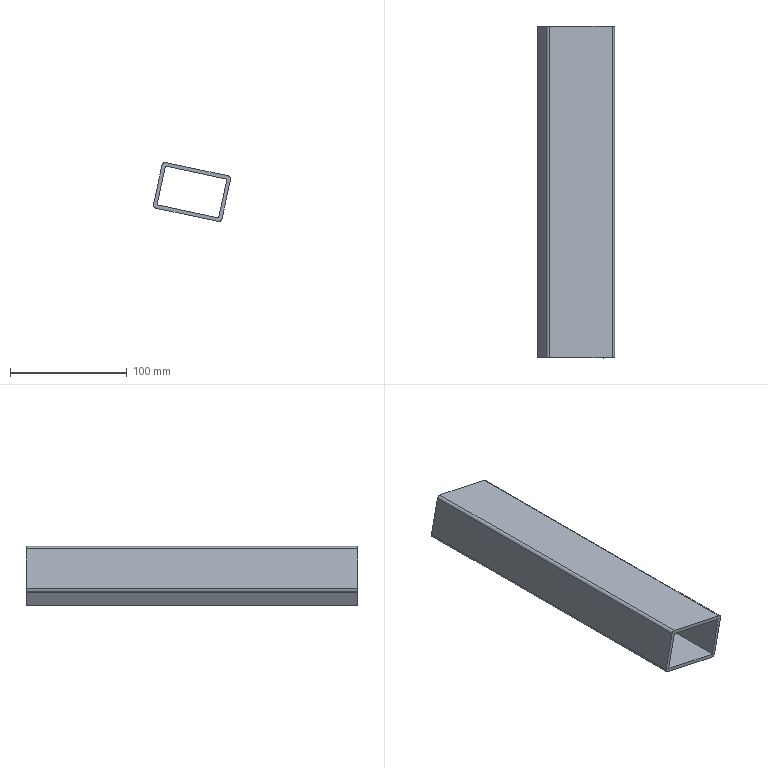Part | STEP file | support fixing frame | 1 solid | 14 faces | box 66.075 x 284.5 x 50.67 mm | volume 158932 mm3 | plane 10 | cylinder 4 | commonest cylinder face diameters 5 x4
STEP:
#1=CARTESIAN_POINT('',(0.,0.,0.));
#2=DIRECTION('',(0.,0.,1.));
#3=DIRECTION('',(1.,0.,0.));
#4=AXIS2_PLACEMENT_3D('',#1,#2,#3);
#5=CARTESIAN_POINT('',(1767.422,305.,-292.036));
#6=VERTEX_POINT('',#5);
#7=CARTESIAN_POINT('',(1770.387,305.,-290.111));
#8=VERTEX_POINT('',#7);
#9=CARTESIAN_POINT('',(1769.867,305.,-292.556));
#10=DIRECTION('',(0.,1.,0.));
#11=DIRECTION('',(0.,0.,-1.));
#12=AXIS2_PLACEMENT_3D('',#9,#10,#11);
#13=CIRCLE('',#12,2.5);
#14=CARTESIAN_POINT('',(1769.867,0.,-292.556));
#15=DIRECTION('',(0.,1.,0.));
#16=DIRECTION('',(1.,0.,0.));
#17=AXIS2_PLACEMENT_3D('',#14,#15,#16);
#18=CYLINDRICAL_SURFACE('',#17,2.5);
#19=CARTESIAN_POINT('',(1.571,305.));
#20=DIRECTION('',(1.,0.));
#21=VECTOR('',#20,1.);
#22=LINE('',#19,#21);
#23=(GEOMETRIC_REPRESENTATION_CONTEXT(2)PARAMETRIC_REPRESENTATION_CONTEXT()REPRESENTATION_CONTEXT('',''));
#24=DEFINITIONAL_REPRESENTATION('',(#22),#23);
#25=PCURVE('',#18,#24);
#26=CARTESIAN_POINT('',(1655.76,305.,323.083));
#27=DIRECTION('',(0.,-1.,0.));
#28=DIRECTION('',(0.,0.,1.));
#29=AXIS2_PLACEMENT_3D('',#26,#27,#28);
#30=PLANE('',#29);
#31=CARTESIAN_POINT('',(-618.139,-114.107));
#32=CARTESIAN_POINT('',(-618.139,-109.777));
#33=CARTESIAN_POINT('',(-614.389,-111.942));
#34=CARTESIAN_POINT('',(-610.639,-114.107));
#35=CARTESIAN_POINT('',(-614.389,-116.272));
#36=CARTESIAN_POINT('',(-618.139,-118.437));
#37=CARTESIAN_POINT('',(-618.139,-114.107));
#38=(BOUNDED_CURVE()B_SPLINE_CURVE(2,(#31,#32,#33,#34,#35,#36,#37),.UNSPECIFIED.,.T.,.F.)B_SPLINE_CURVE_WITH_KNOTS((1,2,2,2,2,1),(-2.094,0.,2.094,4.189,6.283,8.378),.UNSPECIFIED.)CURVE()GEOMETRIC_REPRESENTATION_ITEM()RATIONAL_B_SPLINE_CURVE((1.,0.5,1.,0.5,1.,0.5,1.))REPRESENTATION_ITEM(''));
#39=(GEOMETRIC_REPRESENTATION_CONTEXT(2)PARAMETRIC_REPRESENTATION_CONTEXT()REPRESENTATION_CONTEXT('',''));
#40=DEFINITIONAL_REPRESENTATION('',(#38),#39);
#41=PCURVE('',#30,#40);
#42=SURFACE_CURVE('',#13,(#25,#41),.PCURVE_S1.);
#43=EDGE_CURVE('',#6,#8,#42,.T.);
#44=ORIENTED_EDGE('',*,*,#43,.F.);
#45=CARTESIAN_POINT('',(1767.422,20.5,-292.036));
#46=VERTEX_POINT('',#45);
#47=CARTESIAN_POINT('',(1767.422,386.,-292.036));
#48=DIRECTION('',(0.,1.,0.));
#49=VECTOR('',#48,1.);
#50=LINE('',#47,#49);
#51=CARTESIAN_POINT('',(3.351,386.));
#52=DIRECTION('',(0.,1.));
#53=VECTOR('',#52,1.);
#54=LINE('',#51,#53);
#55=(GEOMETRIC_REPRESENTATION_CONTEXT(2)PARAMETRIC_REPRESENTATION_CONTEXT()REPRESENTATION_CONTEXT('',''));
#56=DEFINITIONAL_REPRESENTATION('',(#54),#55);
#57=PCURVE('',#18,#56);
#58=CARTESIAN_POINT('',(1767.941,386.,-289.591));
#59=DIRECTION('',(0.9781,0.,-0.2079));
#60=DIRECTION('',(0.2079,0.,0.9781));
#61=AXIS2_PLACEMENT_3D('',#58,#59,#60);
#62=PLANE('',#61);
#63=CARTESIAN_POINT('',(-2.5,0.));
#64=DIRECTION('',(0.,-1.));
#65=VECTOR('',#64,1.);
#66=LINE('',#63,#65);
#67=(GEOMETRIC_REPRESENTATION_CONTEXT(2)PARAMETRIC_REPRESENTATION_CONTEXT()REPRESENTATION_CONTEXT('',''));
#68=DEFINITIONAL_REPRESENTATION('',(#66),#67);
#69=PCURVE('',#62,#68);
#70=SURFACE_CURVE('',#50,(#57,#69),.PCURVE_S1.);
#71=EDGE_CURVE('',#46,#6,#70,.T.);
#72=ORIENTED_EDGE('',*,*,#71,.F.);
#73=CARTESIAN_POINT('',(1770.387,20.5,-290.111));
#74=VERTEX_POINT('',#73);
#75=CARTESIAN_POINT('',(1769.867,20.5,-292.556));
#76=DIRECTION('',(0.,-1.,0.));
#77=DIRECTION('',(-1.,0.,0.));
#78=AXIS2_PLACEMENT_3D('',#75,#76,#77);
#79=CIRCLE('',#78,2.5);
#80=CARTESIAN_POINT('',(9.425,20.5));
#81=DIRECTION('',(-1.,0.));
#82=VECTOR('',#81,1.);
#83=LINE('',#80,#82);
#84=(GEOMETRIC_REPRESENTATION_CONTEXT(2)PARAMETRIC_REPRESENTATION_CONTEXT()REPRESENTATION_CONTEXT('',''));
#85=DEFINITIONAL_REPRESENTATION('',(#83),#84);
#86=PCURVE('',#18,#85);
#87=CARTESIAN_POINT('',(1767.941,20.5,-289.591));
#88=DIRECTION('',(0.,1.,0.));
#89=DIRECTION('',(1.,0.,0.));
#90=AXIS2_PLACEMENT_3D('',#87,#88,#89);
#91=PLANE('',#90);
#92=CARTESIAN_POINT('',(-0.5744,2.965));
#93=CARTESIAN_POINT('',(-0.5744,7.295));
#94=CARTESIAN_POINT('',(3.176,5.13));
#95=CARTESIAN_POINT('',(6.926,2.965));
#96=CARTESIAN_POINT('',(3.176,0.8001));
#97=CARTESIAN_POINT('',(-0.5744,-1.365));
#98=CARTESIAN_POINT('',(-0.5744,2.965));
#99=(BOUNDED_CURVE()B_SPLINE_CURVE(2,(#92,#93,#94,#95,#96,#97,#98),.UNSPECIFIED.,.T.,.F.)B_SPLINE_CURVE_WITH_KNOTS((1,2,2,2,2,1),(-2.094,0.,2.094,4.189,6.283,8.378),.UNSPECIFIED.)CURVE()GEOMETRIC_REPRESENTATION_ITEM()RATIONAL_B_SPLINE_CURVE((1.,0.5,1.,0.5,1.,0.5,1.))REPRESENTATION_ITEM(''));
#100=(GEOMETRIC_REPRESENTATION_CONTEXT(2)PARAMETRIC_REPRESENTATION_CONTEXT()REPRESENTATION_CONTEXT('',''));
#101=DEFINITIONAL_REPRESENTATION('',(#99),#100);
#102=PCURVE('',#91,#101);
#103=SURFACE_CURVE('',#79,(#86,#102),.PCURVE_S1.);
#104=EDGE_CURVE('',#74,#46,#103,.T.);
#105=ORIENTED_EDGE('',*,*,#104,.F.);
#106=CARTESIAN_POINT('',(1770.387,20.5,-290.111));
#107=DIRECTION('',(0.,-1.,0.));
#108=VECTOR('',#107,1.);
#109=LINE('',#106,#108);
#110=CARTESIAN_POINT('',(4.922,20.5));
#111=DIRECTION('',(0.,-1.));
#112=VECTOR('',#111,1.);
#113=LINE('',#110,#112);
#114=(GEOMETRIC_REPRESENTATION_CONTEXT(2)PARAMETRIC_REPRESENTATION_CONTEXT()REPRESENTATION_CONTEXT('',''));
#115=DEFINITIONAL_REPRESENTATION('',(#113),#114);
#116=PCURVE('',#18,#115);
#117=CARTESIAN_POINT('',(17.53,0.,82.471));
#118=DIRECTION('',(0.2079,0.,0.9781));
#119=DIRECTION('',(-0.9781,0.,0.2079));
#120=AXIS2_PLACEMENT_3D('',#117,#118,#119);
#121=PLANE('',#120);
#122=CARTESIAN_POINT('',(-1792.017,-20.5));
#123=DIRECTION('',(0.,1.));
#124=VECTOR('',#123,1.);
#125=LINE('',#122,#124);
#126=(GEOMETRIC_REPRESENTATION_CONTEXT(2)PARAMETRIC_REPRESENTATION_CONTEXT()REPRESENTATION_CONTEXT('',''));
#127=DEFINITIONAL_REPRESENTATION('',(#125),#126);
#128=PCURVE('',#121,#127);
#129=SURFACE_CURVE('',#109,(#116,#128),.PCURVE_S1.);
#130=EDGE_CURVE('',#8,#74,#129,.T.);
#131=ORIENTED_EDGE('',*,*,#130,.F.);
#132=EDGE_LOOP('',(#44,#72,#105,#131));
#133=FACE_BOUND('',#132,.T.);
#134=ADVANCED_FACE('',(#133),#18,.T.);
#135=CARTESIAN_POINT('',(1826.11,20.5,-304.511));
#136=VERTEX_POINT('',#135);
#137=CARTESIAN_POINT('',(1824.185,20.5,-301.546));
#138=VERTEX_POINT('',#137);
#139=CARTESIAN_POINT('',(1823.665,20.5,-303.991));
#140=DIRECTION('',(0.,-1.,0.));
#141=DIRECTION('',(-1.,0.,0.));
#142=AXIS2_PLACEMENT_3D('',#139,#140,#141);
#143=CIRCLE('',#142,2.5);
#144=CARTESIAN_POINT('',(1823.665,0.,-303.991));
#145=DIRECTION('',(0.,-1.,0.));
#146=DIRECTION('',(0.,0.,1.));
#147=AXIS2_PLACEMENT_3D('',#144,#145,#146);
#148=CYLINDRICAL_SURFACE('',#147,2.5);
#149=CARTESIAN_POINT('',(1.571,-20.5));
#150=DIRECTION('',(1.,0.));
#151=VECTOR('',#150,1.);
#152=LINE('',#149,#151);
#153=(GEOMETRIC_REPRESENTATION_CONTEXT(2)PARAMETRIC_REPRESENTATION_CONTEXT()REPRESENTATION_CONTEXT('',''));
#154=DEFINITIONAL_REPRESENTATION('',(#152),#153);
#155=PCURVE('',#148,#154);
#156=CARTESIAN_POINT('',(53.224,14.4));
#157=CARTESIAN_POINT('',(53.224,18.73));
#158=CARTESIAN_POINT('',(56.974,16.565));
#159=CARTESIAN_POINT('',(60.724,14.4));
#160=CARTESIAN_POINT('',(56.974,12.235));
#161=CARTESIAN_POINT('',(53.224,10.07));
#162=CARTESIAN_POINT('',(53.224,14.4));
#163=(BOUNDED_CURVE()B_SPLINE_CURVE(2,(#156,#157,#158,#159,#160,#161,#162),.UNSPECIFIED.,.T.,.F.)B_SPLINE_CURVE_WITH_KNOTS((1,2,2,2,2,1),(-2.094,0.,2.094,4.189,6.283,8.378),.UNSPECIFIED.)CURVE()GEOMETRIC_REPRESENTATION_ITEM()RATIONAL_B_SPLINE_CURVE((1.,0.5,1.,0.5,1.,0.5,1.))REPRESENTATION_ITEM(''));
#164=(GEOMETRIC_REPRESENTATION_CONTEXT(2)PARAMETRIC_REPRESENTATION_CONTEXT()REPRESENTATION_CONTEXT('',''));
#165=DEFINITIONAL_REPRESENTATION('',(#163),#164);
#166=PCURVE('',#91,#165);
#167=SURFACE_CURVE('',#143,(#155,#166),.PCURVE_S1.);
#168=EDGE_CURVE('',#136,#138,#167,.T.);
#169=ORIENTED_EDGE('',*,*,#168,.F.);
#170=CARTESIAN_POINT('',(1826.11,305.,-304.511));
#171=VERTEX_POINT('',#170);
#172=CARTESIAN_POINT('',(1826.11,20.5,-304.511));
#173=DIRECTION('',(0.,-1.,0.));
#174=VECTOR('',#173,1.);
#175=LINE('',#172,#174);
#176=CARTESIAN_POINT('',(4.503,-20.5));
#177=DIRECTION('',(0.,1.));
#178=VECTOR('',#177,1.);
#179=LINE('',#176,#178);
#180=(GEOMETRIC_REPRESENTATION_CONTEXT(2)PARAMETRIC_REPRESENTATION_CONTEXT()REPRESENTATION_CONTEXT('',''));
#181=DEFINITIONAL_REPRESENTATION('',(#179),#180);
#182=PCURVE('',#148,#181);
#183=CARTESIAN_POINT('',(1826.63,20.5,-302.066));
#184=DIRECTION('',(-0.9781,0.,0.2079));
#185=DIRECTION('',(-0.2079,0.,-0.9781));
#186=AXIS2_PLACEMENT_3D('',#183,#184,#185);
#187=PLANE('',#186);
#188=CARTESIAN_POINT('',(2.5,0.));
#189=DIRECTION('',(0.,1.));
#190=VECTOR('',#189,1.);
#191=LINE('',#188,#190);
#192=(GEOMETRIC_REPRESENTATION_CONTEXT(2)PARAMETRIC_REPRESENTATION_CONTEXT()REPRESENTATION_CONTEXT('',''));
#193=DEFINITIONAL_REPRESENTATION('',(#191),#192);
#194=PCURVE('',#187,#193);
#195=SURFACE_CURVE('',#175,(#182,#194),.PCURVE_S1.);
#196=EDGE_CURVE('',#171,#136,#195,.T.);
#197=ORIENTED_EDGE('',*,*,#196,.F.);
#198=CARTESIAN_POINT('',(1824.185,305.,-301.546));
#199=VERTEX_POINT('',#198);
#200=CARTESIAN_POINT('',(1823.665,305.,-303.991));
#201=DIRECTION('',(0.,1.,0.));
#202=DIRECTION('',(0.,0.,-1.));
#203=AXIS2_PLACEMENT_3D('',#200,#201,#202);
#204=CIRCLE('',#203,2.5);
#205=CARTESIAN_POINT('',(9.425,-305.));
#206=DIRECTION('',(-1.,0.));
#207=VECTOR('',#206,1.);
#208=LINE('',#205,#207);
#209=(GEOMETRIC_REPRESENTATION_CONTEXT(2)PARAMETRIC_REPRESENTATION_CONTEXT()REPRESENTATION_CONTEXT('',''));
#210=DEFINITIONAL_REPRESENTATION('',(#208),#209);
#211=PCURVE('',#148,#210);
#212=CARTESIAN_POINT('',(-629.574,-167.905));
#213=CARTESIAN_POINT('',(-629.574,-163.575));
#214=CARTESIAN_POINT('',(-625.824,-165.74));
#215=CARTESIAN_POINT('',(-622.074,-167.905));
#216=CARTESIAN_POINT('',(-625.824,-170.07));
#217=CARTESIAN_POINT('',(-629.574,-172.235));
#218=CARTESIAN_POINT('',(-629.574,-167.905));
#219=(BOUNDED_CURVE()B_SPLINE_CURVE(2,(#212,#213,#214,#215,#216,#217,#218),.UNSPECIFIED.,.T.,.F.)B_SPLINE_CURVE_WITH_KNOTS((1,2,2,2,2,1),(-2.094,0.,2.094,4.189,6.283,8.378),.UNSPECIFIED.)CURVE()GEOMETRIC_REPRESENTATION_ITEM()RATIONAL_B_SPLINE_CURVE((1.,0.5,1.,0.5,1.,0.5,1.))REPRESENTATION_ITEM(''));
#220=(GEOMETRIC_REPRESENTATION_CONTEXT(2)PARAMETRIC_REPRESENTATION_CONTEXT()REPRESENTATION_CONTEXT('',''));
#221=DEFINITIONAL_REPRESENTATION('',(#219),#220);
#222=PCURVE('',#30,#221);
#223=SURFACE_CURVE('',#204,(#211,#222),.PCURVE_S1.);
#224=EDGE_CURVE('',#199,#171,#223,.T.);
#225=ORIENTED_EDGE('',*,*,#224,.F.);
#226=CARTESIAN_POINT('',(1824.185,386.,-301.546));
#227=DIRECTION('',(0.,1.,0.));
#228=VECTOR('',#227,1.);
#229=LINE('',#226,#228);
#230=CARTESIAN_POINT('',(6.074,-386.));
#231=DIRECTION('',(0.,-1.));
#232=VECTOR('',#231,1.);
#233=LINE('',#230,#232);
#234=(GEOMETRIC_REPRESENTATION_CONTEXT(2)PARAMETRIC_REPRESENTATION_CONTEXT()REPRESENTATION_CONTEXT('',''));
#235=DEFINITIONAL_REPRESENTATION('',(#233),#234);
#236=PCURVE('',#148,#235);
#237=CARTESIAN_POINT('',(-1847.017,-386.));
#238=DIRECTION('',(0.,-1.));
#239=VECTOR('',#238,1.);
#240=LINE('',#237,#239);
#241=(GEOMETRIC_REPRESENTATION_CONTEXT(2)PARAMETRIC_REPRESENTATION_CONTEXT()REPRESENTATION_CONTEXT('',''));
#242=DEFINITIONAL_REPRESENTATION('',(#240),#241);
#243=PCURVE('',#121,#242);
#244=SURFACE_CURVE('',#229,(#236,#243),.PCURVE_S1.);
#245=EDGE_CURVE('',#138,#199,#244,.T.);
#246=ORIENTED_EDGE('',*,*,#245,.F.);
#247=EDGE_LOOP('',(#169,#197,#225,#246));
#248=FACE_BOUND('',#247,.T.);
#249=ADVANCED_FACE('',(#248),#148,.T.);
#250=CARTESIAN_POINT('',(1762.07,305.,-329.237));
#251=VERTEX_POINT('',#250);
#252=CARTESIAN_POINT('',(1760.145,305.,-326.271));
#253=VERTEX_POINT('',#252);
#254=CARTESIAN_POINT('',(1762.59,305.,-326.791));
#255=DIRECTION('',(0.,1.,0.));
#256=DIRECTION('',(0.,0.,-1.));
#257=AXIS2_PLACEMENT_3D('',#254,#255,#256);
#258=CIRCLE('',#257,2.5);
#259=CARTESIAN_POINT('',(1762.59,386.,-326.791));
#260=DIRECTION('',(0.,-1.,0.));
#261=DIRECTION('',(-1.,0.,0.));
#262=AXIS2_PLACEMENT_3D('',#259,#260,#261);
#263=CYLINDRICAL_SURFACE('',#262,2.5);
#264=CARTESIAN_POINT('',(1.571,81.));
#265=DIRECTION('',(-1.,0.));
#266=VECTOR('',#265,1.);
#267=LINE('',#264,#266);
#268=(GEOMETRIC_REPRESENTATION_CONTEXT(2)PARAMETRIC_REPRESENTATION_CONTEXT()REPRESENTATION_CONTEXT('',''));
#269=DEFINITIONAL_REPRESENTATION('',(#267),#268);
#270=PCURVE('',#263,#269);
#271=CARTESIAN_POINT('',(-652.374,-106.83));
#272=CARTESIAN_POINT('',(-652.374,-102.5));
#273=CARTESIAN_POINT('',(-648.624,-104.665));
#274=CARTESIAN_POINT('',(-644.874,-106.83));
#275=CARTESIAN_POINT('',(-648.624,-108.995));
#276=CARTESIAN_POINT('',(-652.374,-111.16));
#277=CARTESIAN_POINT('',(-652.374,-106.83));
#278=(BOUNDED_CURVE()B_SPLINE_CURVE(2,(#271,#272,#273,#274,#275,#276,#277),.UNSPECIFIED.,.T.,.F.)B_SPLINE_CURVE_WITH_KNOTS((1,2,2,2,2,1),(-2.094,0.,2.094,4.189,6.283,8.378),.UNSPECIFIED.)CURVE()GEOMETRIC_REPRESENTATION_ITEM()RATIONAL_B_SPLINE_CURVE((1.,0.5,1.,0.5,1.,0.5,1.))REPRESENTATION_ITEM(''));
#279=(GEOMETRIC_REPRESENTATION_CONTEXT(2)PARAMETRIC_REPRESENTATION_CONTEXT()REPRESENTATION_CONTEXT('',''));
#280=DEFINITIONAL_REPRESENTATION('',(#278),#279);
#281=PCURVE('',#30,#280);
#282=SURFACE_CURVE('',#258,(#270,#281),.PCURVE_S1.);
#283=EDGE_CURVE('',#251,#253,#282,.T.);
#284=ORIENTED_EDGE('',*,*,#283,.F.);
#285=CARTESIAN_POINT('',(1762.07,20.5,-329.237));
#286=VERTEX_POINT('',#285);
#287=CARTESIAN_POINT('',(1762.07,0.,-329.237));
#288=DIRECTION('',(0.,1.,0.));
#289=VECTOR('',#288,1.);
#290=LINE('',#287,#289);
#291=CARTESIAN_POINT('',(1.361,386.));
#292=DIRECTION('',(0.,-1.));
#293=VECTOR('',#292,1.);
#294=LINE('',#291,#293);
#295=(GEOMETRIC_REPRESENTATION_CONTEXT(2)PARAMETRIC_REPRESENTATION_CONTEXT()REPRESENTATION_CONTEXT('',''));
#296=DEFINITIONAL_REPRESENTATION('',(#294),#295);
#297=PCURVE('',#263,#296);
#298=CARTESIAN_POINT('',(9.213,0.,43.345));
#299=DIRECTION('',(0.2079,0.,0.9781));
#300=DIRECTION('',(-0.9781,0.,0.2079));
#301=AXIS2_PLACEMENT_3D('',#298,#299,#300);
#302=PLANE('',#301);
#303=CARTESIAN_POINT('',(-1792.017,0.));
#304=DIRECTION('',(0.,-1.));
#305=VECTOR('',#304,1.);
#306=LINE('',#303,#305);
#307=(GEOMETRIC_REPRESENTATION_CONTEXT(2)PARAMETRIC_REPRESENTATION_CONTEXT()REPRESENTATION_CONTEXT('',''));
#308=DEFINITIONAL_REPRESENTATION('',(#306),#307);
#309=PCURVE('',#302,#308);
#310=SURFACE_CURVE('',#290,(#297,#309),.PCURVE_S1.);
#311=EDGE_CURVE('',#286,#251,#310,.T.);
#312=ORIENTED_EDGE('',*,*,#311,.F.);
#313=CARTESIAN_POINT('',(1760.145,20.5,-326.271));
#314=VERTEX_POINT('',#313);
#315=CARTESIAN_POINT('',(1762.59,20.5,-326.791));
#316=DIRECTION('',(0.,-1.,0.));
#317=DIRECTION('',(-1.,0.,0.));
#318=AXIS2_PLACEMENT_3D('',#315,#316,#317);
#319=CIRCLE('',#318,2.5);
#320=CARTESIAN_POINT('',(-6.283,365.5));
#321=DIRECTION('',(1.,0.));
#322=VECTOR('',#321,1.);
#323=LINE('',#320,#322);
#324=(GEOMETRIC_REPRESENTATION_CONTEXT(2)PARAMETRIC_REPRESENTATION_CONTEXT()REPRESENTATION_CONTEXT('',''));
#325=DEFINITIONAL_REPRESENTATION('',(#323),#324);
#326=PCURVE('',#263,#325);
#327=CARTESIAN_POINT('',(-7.851,37.2));
#328=CARTESIAN_POINT('',(-7.851,41.53));
#329=CARTESIAN_POINT('',(-4.101,39.365));
#330=CARTESIAN_POINT('',(-0.3513,37.2));
#331=CARTESIAN_POINT('',(-4.101,35.035));
#332=CARTESIAN_POINT('',(-7.851,32.87));
#333=CARTESIAN_POINT('',(-7.851,37.2));
#334=(BOUNDED_CURVE()B_SPLINE_CURVE(2,(#327,#328,#329,#330,#331,#332,#333),.UNSPECIFIED.,.T.,.F.)B_SPLINE_CURVE_WITH_KNOTS((1,2,2,2,2,1),(-2.094,0.,2.094,4.189,6.283,8.378),.UNSPECIFIED.)CURVE()GEOMETRIC_REPRESENTATION_ITEM()RATIONAL_B_SPLINE_CURVE((1.,0.5,1.,0.5,1.,0.5,1.))REPRESENTATION_ITEM(''));
#335=(GEOMETRIC_REPRESENTATION_CONTEXT(2)PARAMETRIC_REPRESENTATION_CONTEXT()REPRESENTATION_CONTEXT('',''));
#336=DEFINITIONAL_REPRESENTATION('',(#334),#335);
#337=PCURVE('',#91,#336);
#338=SURFACE_CURVE('',#319,(#326,#337),.PCURVE_S1.);
#339=EDGE_CURVE('',#314,#286,#338,.T.);
#340=ORIENTED_EDGE('',*,*,#339,.F.);
#341=CARTESIAN_POINT('',(1760.145,386.,-326.271));
#342=DIRECTION('',(0.,-1.,0.));
#343=VECTOR('',#342,1.);
#344=LINE('',#341,#343);
#345=CARTESIAN_POINT('',(-0.2094,0.));
#346=DIRECTION('',(0.,1.));
#347=VECTOR('',#346,1.);
#348=LINE('',#345,#347);
#349=(GEOMETRIC_REPRESENTATION_CONTEXT(2)PARAMETRIC_REPRESENTATION_CONTEXT()REPRESENTATION_CONTEXT('',''));
#350=DEFINITIONAL_REPRESENTATION('',(#348),#349);
#351=PCURVE('',#263,#350);
#352=CARTESIAN_POINT('',(-37.5,0.));
#353=DIRECTION('',(0.,1.));
#354=VECTOR('',#353,1.);
#355=LINE('',#352,#354);
#356=(GEOMETRIC_REPRESENTATION_CONTEXT(2)PARAMETRIC_REPRESENTATION_CONTEXT()REPRESENTATION_CONTEXT('',''));
#357=DEFINITIONAL_REPRESENTATION('',(#355),#356);
#358=PCURVE('',#62,#357);
#359=SURFACE_CURVE('',#344,(#351,#358),.PCURVE_S1.);
#360=EDGE_CURVE('',#253,#314,#359,.T.);
#361=ORIENTED_EDGE('',*,*,#360,.F.);
#362=EDGE_LOOP('',(#284,#312,#340,#361));
#363=FACE_BOUND('',#362,.T.);
#364=ADVANCED_FACE('',(#363),#263,.T.);
#365=CARTESIAN_POINT('',(1815.868,20.5,-340.672));
#366=VERTEX_POINT('',#365);
#367=CARTESIAN_POINT('',(1818.833,20.5,-338.746));
#368=VERTEX_POINT('',#367);
#369=CARTESIAN_POINT('',(1816.388,20.5,-338.226));
#370=DIRECTION('',(0.,-1.,0.));
#371=DIRECTION('',(-1.,0.,0.));
#372=AXIS2_PLACEMENT_3D('',#369,#370,#371);
#373=CIRCLE('',#372,2.5);
#374=CARTESIAN_POINT('',(1816.388,20.5,-338.226));
#375=DIRECTION('',(0.,1.,0.));
#376=DIRECTION('',(0.,0.,-1.));
#377=AXIS2_PLACEMENT_3D('',#374,#375,#376);
#378=CYLINDRICAL_SURFACE('',#377,2.5);
#379=CARTESIAN_POINT('',(7.854,0.));
#380=DIRECTION('',(-1.,0.));
#381=VECTOR('',#380,1.);
#382=LINE('',#379,#381);
#383=(GEOMETRIC_REPRESENTATION_CONTEXT(2)PARAMETRIC_REPRESENTATION_CONTEXT()REPRESENTATION_CONTEXT('',''));
#384=DEFINITIONAL_REPRESENTATION('',(#382),#383);
#385=PCURVE('',#378,#384);
#386=CARTESIAN_POINT('',(45.947,48.635));
#387=CARTESIAN_POINT('',(45.947,52.966));
#388=CARTESIAN_POINT('',(49.697,50.801));
#389=CARTESIAN_POINT('',(53.447,48.635));
#390=CARTESIAN_POINT('',(49.697,46.47));
#391=CARTESIAN_POINT('',(45.947,44.305));
#392=CARTESIAN_POINT('',(45.947,48.635));
#393=(BOUNDED_CURVE()B_SPLINE_CURVE(2,(#386,#387,#388,#389,#390,#391,#392),.UNSPECIFIED.,.T.,.F.)B_SPLINE_CURVE_WITH_KNOTS((1,2,2,2,2,1),(-2.094,0.,2.094,4.189,6.283,8.378),.UNSPECIFIED.)CURVE()GEOMETRIC_REPRESENTATION_ITEM()RATIONAL_B_SPLINE_CURVE((1.,0.5,1.,0.5,1.,0.5,1.))REPRESENTATION_ITEM(''));
#394=(GEOMETRIC_REPRESENTATION_CONTEXT(2)PARAMETRIC_REPRESENTATION_CONTEXT()REPRESENTATION_CONTEXT('',''));
#395=DEFINITIONAL_REPRESENTATION('',(#393),#394);
#396=PCURVE('',#91,#395);
#397=SURFACE_CURVE('',#373,(#385,#396),.PCURVE_S1.);
#398=EDGE_CURVE('',#366,#368,#397,.T.);
#399=ORIENTED_EDGE('',*,*,#398,.F.);
#400=CARTESIAN_POINT('',(1815.868,305.,-340.672));
#401=VERTEX_POINT('',#400);
#402=CARTESIAN_POINT('',(1815.868,0.,-340.672));
#403=DIRECTION('',(0.,-1.,0.));
#404=VECTOR('',#403,1.);
#405=LINE('',#402,#404);
#406=CARTESIAN_POINT('',(6.493,-20.5));
#407=DIRECTION('',(0.,-1.));
#408=VECTOR('',#407,1.);
#409=LINE('',#406,#408);
#410=(GEOMETRIC_REPRESENTATION_CONTEXT(2)PARAMETRIC_REPRESENTATION_CONTEXT()REPRESENTATION_CONTEXT('',''));
#411=DEFINITIONAL_REPRESENTATION('',(#409),#410);
#412=PCURVE('',#378,#411);
#413=CARTESIAN_POINT('',(-1847.017,0.));
#414=DIRECTION('',(0.,1.));
#415=VECTOR('',#414,1.);
#416=LINE('',#413,#415);
#417=(GEOMETRIC_REPRESENTATION_CONTEXT(2)PARAMETRIC_REPRESENTATION_CONTEXT()REPRESENTATION_CONTEXT('',''));
#418=DEFINITIONAL_REPRESENTATION('',(#416),#417);
#419=PCURVE('',#302,#418);
#420=SURFACE_CURVE('',#405,(#412,#419),.PCURVE_S1.);
#421=EDGE_CURVE('',#401,#366,#420,.T.);
#422=ORIENTED_EDGE('',*,*,#421,.F.);
#423=CARTESIAN_POINT('',(1818.833,305.,-338.746));
#424=VERTEX_POINT('',#423);
#425=CARTESIAN_POINT('',(1816.388,305.,-338.226));
#426=DIRECTION('',(0.,1.,0.));
#427=DIRECTION('',(0.,0.,-1.));
#428=AXIS2_PLACEMENT_3D('',#425,#426,#427);
#429=CIRCLE('',#428,2.5);
#430=CARTESIAN_POINT('',(0.,284.5));
#431=DIRECTION('',(1.,0.));
#432=VECTOR('',#431,1.);
#433=LINE('',#430,#432);
#434=(GEOMETRIC_REPRESENTATION_CONTEXT(2)PARAMETRIC_REPRESENTATION_CONTEXT()REPRESENTATION_CONTEXT('',''));
#435=DEFINITIONAL_REPRESENTATION('',(#433),#434);
#436=PCURVE('',#378,#435);
#437=CARTESIAN_POINT('',(-663.809,-160.628));
#438=CARTESIAN_POINT('',(-663.809,-156.298));
#439=CARTESIAN_POINT('',(-660.059,-158.463));
#440=CARTESIAN_POINT('',(-656.309,-160.628));
#441=CARTESIAN_POINT('',(-660.059,-162.794));
#442=CARTESIAN_POINT('',(-663.809,-164.959));
#443=CARTESIAN_POINT('',(-663.809,-160.628));
#444=(BOUNDED_CURVE()B_SPLINE_CURVE(2,(#437,#438,#439,#440,#441,#442,#443),.UNSPECIFIED.,.T.,.F.)B_SPLINE_CURVE_WITH_KNOTS((1,2,2,2,2,1),(-2.094,0.,2.094,4.189,6.283,8.378),.UNSPECIFIED.)CURVE()GEOMETRIC_REPRESENTATION_ITEM()RATIONAL_B_SPLINE_CURVE((1.,0.5,1.,0.5,1.,0.5,1.))REPRESENTATION_ITEM(''));
#445=(GEOMETRIC_REPRESENTATION_CONTEXT(2)PARAMETRIC_REPRESENTATION_CONTEXT()REPRESENTATION_CONTEXT('',''));
#446=DEFINITIONAL_REPRESENTATION('',(#444),#445);
#447=PCURVE('',#30,#446);
#448=SURFACE_CURVE('',#429,(#436,#447),.PCURVE_S1.);
#449=EDGE_CURVE('',#424,#401,#448,.T.);
#450=ORIENTED_EDGE('',*,*,#449,.F.);
#451=CARTESIAN_POINT('',(1818.833,20.5,-338.746));
#452=DIRECTION('',(0.,1.,0.));
#453=VECTOR('',#452,1.);
#454=LINE('',#451,#453);
#455=CARTESIAN_POINT('',(4.922,0.));
#456=DIRECTION('',(0.,1.));
#457=VECTOR('',#456,1.);
#458=LINE('',#455,#457);
#459=(GEOMETRIC_REPRESENTATION_CONTEXT(2)PARAMETRIC_REPRESENTATION_CONTEXT()REPRESENTATION_CONTEXT('',''));
#460=DEFINITIONAL_REPRESENTATION('',(#458),#459);
#461=PCURVE('',#378,#460);
#462=CARTESIAN_POINT('',(37.5,0.));
#463=DIRECTION('',(0.,-1.));
#464=VECTOR('',#463,1.);
#465=LINE('',#462,#464);
#466=(GEOMETRIC_REPRESENTATION_CONTEXT(2)PARAMETRIC_REPRESENTATION_CONTEXT()REPRESENTATION_CONTEXT('',''));
#467=DEFINITIONAL_REPRESENTATION('',(#465),#466);
#468=PCURVE('',#187,#467);
#469=SURFACE_CURVE('',#454,(#461,#468),.PCURVE_S1.);
#470=EDGE_CURVE('',#368,#424,#469,.T.);
#471=ORIENTED_EDGE('',*,*,#470,.F.);
#472=EDGE_LOOP('',(#399,#422,#450,#471));
#473=FACE_BOUND('',#472,.T.);
#474=ADVANCED_FACE('',(#473),#378,.T.);
#475=CARTESIAN_POINT('',(1763.183,305.,-326.406));
#476=VERTEX_POINT('',#475);
#477=CARTESIAN_POINT('',(1763.183,20.5,-326.406));
#478=VERTEX_POINT('',#477);
#479=CARTESIAN_POINT('',(1763.183,386.,-326.406));
#480=DIRECTION('',(0.,-1.,0.));
#481=VECTOR('',#480,1.);
#482=LINE('',#479,#481);
#483=CARTESIAN_POINT('',(9.837,0.,46.279));
#484=DIRECTION('',(0.2079,0.,0.9781));
#485=DIRECTION('',(-0.9781,0.,0.2079));
#486=AXIS2_PLACEMENT_3D('',#483,#484,#485);
#487=PLANE('',#486);
#488=CARTESIAN_POINT('',(-1792.517,-386.));
#489=DIRECTION('',(0.,1.));
#490=VECTOR('',#489,1.);
#491=LINE('',#488,#490);
#492=(GEOMETRIC_REPRESENTATION_CONTEXT(2)PARAMETRIC_REPRESENTATION_CONTEXT()REPRESENTATION_CONTEXT('',''));
#493=DEFINITIONAL_REPRESENTATION('',(#491),#492);
#494=PCURVE('',#487,#493);
#495=CARTESIAN_POINT('',(1770.876,386.,-290.215));
#496=DIRECTION('',(0.9781,0.,-0.2079));
#497=DIRECTION('',(0.2079,0.,0.9781));
#498=AXIS2_PLACEMENT_3D('',#495,#496,#497);
#499=PLANE('',#498);
#500=CARTESIAN_POINT('',(-37.,0.));
#501=DIRECTION('',(0.,1.));
#502=VECTOR('',#501,1.);
#503=LINE('',#500,#502);
#504=(GEOMETRIC_REPRESENTATION_CONTEXT(2)PARAMETRIC_REPRESENTATION_CONTEXT()REPRESENTATION_CONTEXT('',''));
#505=DEFINITIONAL_REPRESENTATION('',(#503),#504);
#506=PCURVE('',#499,#505);
#507=SURFACE_CURVE('',#482,(#494,#506),.PCURVE_S1.);
#508=EDGE_CURVE('',#476,#478,#507,.T.);
#509=ORIENTED_EDGE('',*,*,#508,.T.);
#510=CARTESIAN_POINT('',(1816.003,20.5,-337.633));
#511=VERTEX_POINT('',#510);
#512=CARTESIAN_POINT('',(1760.249,20.5,-325.782));
#513=DIRECTION('',(0.9781,0.,-0.2079));
#514=VECTOR('',#513,1.);
#515=LINE('',#512,#514);
#516=CARTESIAN_POINT('',(-1789.517,-20.5));
#517=DIRECTION('',(-1.,0.));
#518=VECTOR('',#517,1.);
#519=LINE('',#516,#518);
#520=(GEOMETRIC_REPRESENTATION_CONTEXT(2)PARAMETRIC_REPRESENTATION_CONTEXT()REPRESENTATION_CONTEXT('',''));
#521=DEFINITIONAL_REPRESENTATION('',(#519),#520);
#522=PCURVE('',#487,#521);
#523=CARTESIAN_POINT('',(-7.693,36.191));
#524=DIRECTION('',(0.9781,0.2079));
#525=VECTOR('',#524,1.);
#526=LINE('',#523,#525);
#527=(GEOMETRIC_REPRESENTATION_CONTEXT(2)PARAMETRIC_REPRESENTATION_CONTEXT()REPRESENTATION_CONTEXT('',''));
#528=DEFINITIONAL_REPRESENTATION('',(#526),#527);
#529=PCURVE('',#91,#528);
#530=SURFACE_CURVE('',#515,(#522,#529),.PCURVE_S1.);
#531=EDGE_CURVE('',#478,#511,#530,.T.);
#532=ORIENTED_EDGE('',*,*,#531,.T.);
#533=CARTESIAN_POINT('',(1816.003,305.,-337.633));
#534=VERTEX_POINT('',#533);
#535=CARTESIAN_POINT('',(1816.003,20.5,-337.633));
#536=DIRECTION('',(0.,1.,0.));
#537=VECTOR('',#536,1.);
#538=LINE('',#535,#537);
#539=CARTESIAN_POINT('',(-1846.517,-20.5));
#540=DIRECTION('',(0.,-1.));
#541=VECTOR('',#540,1.);
#542=LINE('',#539,#541);
#543=(GEOMETRIC_REPRESENTATION_CONTEXT(2)PARAMETRIC_REPRESENTATION_CONTEXT()REPRESENTATION_CONTEXT('',''));
#544=DEFINITIONAL_REPRESENTATION('',(#542),#543);
#545=PCURVE('',#487,#544);
#546=CARTESIAN_POINT('',(1823.696,20.5,-301.442));
#547=DIRECTION('',(-0.9781,0.,0.2079));
#548=DIRECTION('',(-0.2079,0.,-0.9781));
#549=AXIS2_PLACEMENT_3D('',#546,#547,#548);
#550=PLANE('',#549);
#551=CARTESIAN_POINT('',(37.,0.));
#552=DIRECTION('',(0.,-1.));
#553=VECTOR('',#552,1.);
#554=LINE('',#551,#553);
#555=(GEOMETRIC_REPRESENTATION_CONTEXT(2)PARAMETRIC_REPRESENTATION_CONTEXT()REPRESENTATION_CONTEXT('',''));
#556=DEFINITIONAL_REPRESENTATION('',(#554),#555);
#557=PCURVE('',#550,#556);
#558=SURFACE_CURVE('',#538,(#545,#557),.PCURVE_S1.);
#559=EDGE_CURVE('',#511,#534,#558,.T.);
#560=ORIENTED_EDGE('',*,*,#559,.T.);
#561=CARTESIAN_POINT('',(1528.318,305.,-276.484));
#562=DIRECTION('',(-0.9781,0.,0.2079));
#563=VECTOR('',#562,1.);
#564=LINE('',#561,#563);
#565=CARTESIAN_POINT('',(-1552.405,-305.));
#566=DIRECTION('',(1.,0.));
#567=VECTOR('',#566,1.);
#568=LINE('',#565,#567);
#569=(GEOMETRIC_REPRESENTATION_CONTEXT(2)PARAMETRIC_REPRESENTATION_CONTEXT()REPRESENTATION_CONTEXT('',''));
#570=DEFINITIONAL_REPRESENTATION('',(#568),#569);
#571=PCURVE('',#487,#570);
#572=CARTESIAN_POINT('',(-599.567,127.442));
#573=DIRECTION('',(0.2079,0.9781));
#574=VECTOR('',#573,1.);
#575=LINE('',#572,#574);
#576=(GEOMETRIC_REPRESENTATION_CONTEXT(2)PARAMETRIC_REPRESENTATION_CONTEXT()REPRESENTATION_CONTEXT('',''));
#577=DEFINITIONAL_REPRESENTATION('',(#575),#576);
#578=PCURVE('',#30,#577);
#579=SURFACE_CURVE('',#564,(#571,#578),.PCURVE_S1.);
#580=EDGE_CURVE('',#534,#476,#579,.T.);
#581=ORIENTED_EDGE('',*,*,#580,.T.);
#582=EDGE_LOOP('',(#509,#532,#560,#581));
#583=FACE_BOUND('',#582,.T.);
#584=ADVANCED_FACE('',(#583),#487,.T.);
#585=CARTESIAN_POINT('',(1770.252,305.,-293.149));
#586=VERTEX_POINT('',#585);
#587=CARTESIAN_POINT('',(1770.252,20.5,-293.149));
#588=VERTEX_POINT('',#587);
#589=CARTESIAN_POINT('',(1770.252,386.,-293.149));
#590=DIRECTION('',(0.,-1.,0.));
#591=VECTOR('',#590,1.);
#592=LINE('',#589,#591);
#593=CARTESIAN_POINT('',(16.906,0.,79.536));
#594=DIRECTION('',(0.2079,0.,0.9781));
#595=DIRECTION('',(-0.9781,0.,0.2079));
#596=AXIS2_PLACEMENT_3D('',#593,#594,#595);
#597=PLANE('',#596);
#598=CARTESIAN_POINT('',(-1792.517,-386.));
#599=DIRECTION('',(0.,1.));
#600=VECTOR('',#599,1.);
#601=LINE('',#598,#600);
#602=(GEOMETRIC_REPRESENTATION_CONTEXT(2)PARAMETRIC_REPRESENTATION_CONTEXT()REPRESENTATION_CONTEXT('',''));
#603=DEFINITIONAL_REPRESENTATION('',(#601),#602);
#604=PCURVE('',#597,#603);
#605=CARTESIAN_POINT('',(-3.,0.));
#606=DIRECTION('',(0.,1.));
#607=VECTOR('',#606,1.);
#608=LINE('',#605,#607);
#609=(GEOMETRIC_REPRESENTATION_CONTEXT(2)PARAMETRIC_REPRESENTATION_CONTEXT()REPRESENTATION_CONTEXT('',''));
#610=DEFINITIONAL_REPRESENTATION('',(#608),#609);
#611=PCURVE('',#499,#610);
#612=SURFACE_CURVE('',#592,(#604,#611),.PCURVE_S1.);
#613=EDGE_CURVE('',#586,#588,#612,.T.);
#614=ORIENTED_EDGE('',*,*,#613,.F.);
#615=CARTESIAN_POINT('',(1823.072,305.,-304.376));
#616=VERTEX_POINT('',#615);
#617=CARTESIAN_POINT('',(1535.387,305.,-243.227));
#618=DIRECTION('',(-0.9781,0.,0.2079));
#619=VECTOR('',#618,1.);
#620=LINE('',#617,#619);
#621=CARTESIAN_POINT('',(-1552.405,-305.));
#622=DIRECTION('',(1.,0.));
#623=VECTOR('',#622,1.);
#624=LINE('',#621,#623);
#625=(GEOMETRIC_REPRESENTATION_CONTEXT(2)PARAMETRIC_REPRESENTATION_CONTEXT()REPRESENTATION_CONTEXT('',''));
#626=DEFINITIONAL_REPRESENTATION('',(#624),#625);
#627=PCURVE('',#597,#626);
#628=CARTESIAN_POINT('',(-566.31,120.373));
#629=DIRECTION('',(0.2079,0.9781));
#630=VECTOR('',#629,1.);
#631=LINE('',#628,#630);
#632=(GEOMETRIC_REPRESENTATION_CONTEXT(2)PARAMETRIC_REPRESENTATION_CONTEXT()REPRESENTATION_CONTEXT('',''));
#633=DEFINITIONAL_REPRESENTATION('',(#631),#632);
#634=PCURVE('',#30,#633);
#635=SURFACE_CURVE('',#620,(#627,#634),.PCURVE_S1.);
#636=EDGE_CURVE('',#616,#586,#635,.T.);
#637=ORIENTED_EDGE('',*,*,#636,.F.);
#638=CARTESIAN_POINT('',(1823.072,20.5,-304.376));
#639=VERTEX_POINT('',#638);
#640=CARTESIAN_POINT('',(1823.072,20.5,-304.376));
#641=DIRECTION('',(0.,1.,0.));
#642=VECTOR('',#641,1.);
#643=LINE('',#640,#642);
#644=CARTESIAN_POINT('',(-1846.517,-20.5));
#645=DIRECTION('',(0.,-1.));
#646=VECTOR('',#645,1.);
#647=LINE('',#644,#646);
#648=(GEOMETRIC_REPRESENTATION_CONTEXT(2)PARAMETRIC_REPRESENTATION_CONTEXT()REPRESENTATION_CONTEXT('',''));
#649=DEFINITIONAL_REPRESENTATION('',(#647),#648);
#650=PCURVE('',#597,#649);
#651=CARTESIAN_POINT('',(3.,0.));
#652=DIRECTION('',(0.,-1.));
#653=VECTOR('',#652,1.);
#654=LINE('',#651,#653);
#655=(GEOMETRIC_REPRESENTATION_CONTEXT(2)PARAMETRIC_REPRESENTATION_CONTEXT()REPRESENTATION_CONTEXT('',''));
#656=DEFINITIONAL_REPRESENTATION('',(#654),#655);
#657=PCURVE('',#550,#656);
#658=SURFACE_CURVE('',#643,(#650,#657),.PCURVE_S1.);
#659=EDGE_CURVE('',#639,#616,#658,.T.);
#660=ORIENTED_EDGE('',*,*,#659,.F.);
#661=CARTESIAN_POINT('',(1767.318,20.5,-292.525));
#662=DIRECTION('',(0.9781,0.,-0.2079));
#663=VECTOR('',#662,1.);
#664=LINE('',#661,#663);
#665=CARTESIAN_POINT('',(-1789.517,-20.5));
#666=DIRECTION('',(-1.,0.));
#667=VECTOR('',#666,1.);
#668=LINE('',#665,#667);
#669=(GEOMETRIC_REPRESENTATION_CONTEXT(2)PARAMETRIC_REPRESENTATION_CONTEXT()REPRESENTATION_CONTEXT('',''));
#670=DEFINITIONAL_REPRESENTATION('',(#668),#669);
#671=PCURVE('',#597,#670);
#672=CARTESIAN_POINT('',(-0.6237,2.934));
#673=DIRECTION('',(0.9781,0.2079));
#674=VECTOR('',#673,1.);
#675=LINE('',#672,#674);
#676=(GEOMETRIC_REPRESENTATION_CONTEXT(2)PARAMETRIC_REPRESENTATION_CONTEXT()REPRESENTATION_CONTEXT('',''));
#677=DEFINITIONAL_REPRESENTATION('',(#675),#676);
#678=PCURVE('',#91,#677);
#679=SURFACE_CURVE('',#664,(#671,#678),.PCURVE_S1.);
#680=EDGE_CURVE('',#588,#639,#679,.T.);
#681=ORIENTED_EDGE('',*,*,#680,.F.);
#682=EDGE_LOOP('',(#614,#637,#660,#681));
#683=FACE_BOUND('',#682,.T.);
#684=ADVANCED_FACE('',(#683),#597,.F.);
#685=ORIENTED_EDGE('',*,*,#559,.F.);
#686=CARTESIAN_POINT('',(1823.696,20.5,-301.442));
#687=DIRECTION('',(-0.2079,0.,-0.9781));
#688=VECTOR('',#687,1.);
#689=LINE('',#686,#688);
#690=CARTESIAN_POINT('',(0.,0.));
#691=DIRECTION('',(1.,0.));
#692=VECTOR('',#691,1.);
#693=LINE('',#690,#692);
#694=(GEOMETRIC_REPRESENTATION_CONTEXT(2)PARAMETRIC_REPRESENTATION_CONTEXT()REPRESENTATION_CONTEXT('',''));
#695=DEFINITIONAL_REPRESENTATION('',(#693),#694);
#696=PCURVE('',#550,#695);
#697=CARTESIAN_POINT('',(55.754,11.851));
#698=DIRECTION('',(-0.2079,0.9781));
#699=VECTOR('',#698,1.);
#700=LINE('',#697,#699);
#701=(GEOMETRIC_REPRESENTATION_CONTEXT(2)PARAMETRIC_REPRESENTATION_CONTEXT()REPRESENTATION_CONTEXT('',''));
#702=DEFINITIONAL_REPRESENTATION('',(#700),#701);
#703=PCURVE('',#91,#702);
#704=SURFACE_CURVE('',#689,(#696,#703),.PCURVE_S1.);
#705=EDGE_CURVE('',#639,#511,#704,.T.);
#706=ORIENTED_EDGE('',*,*,#705,.F.);
#707=ORIENTED_EDGE('',*,*,#659,.T.);
#708=CARTESIAN_POINT('',(1943.445,305.,261.933));
#709=DIRECTION('',(-0.2079,0.,-0.9781));
#710=VECTOR('',#709,1.);
#711=LINE('',#708,#710);
#712=CARTESIAN_POINT('',(-575.961,-284.5));
#713=DIRECTION('',(1.,0.));
#714=VECTOR('',#713,1.);
#715=LINE('',#712,#714);
#716=(GEOMETRIC_REPRESENTATION_CONTEXT(2)PARAMETRIC_REPRESENTATION_CONTEXT()REPRESENTATION_CONTEXT('',''));
#717=DEFINITIONAL_REPRESENTATION('',(#715),#716);
#718=PCURVE('',#550,#717);
#719=CARTESIAN_POINT('',(-61.149,-287.685));
#720=DIRECTION('',(-0.9781,0.2079));
#721=VECTOR('',#720,1.);
#722=LINE('',#719,#721);
#723=(GEOMETRIC_REPRESENTATION_CONTEXT(2)PARAMETRIC_REPRESENTATION_CONTEXT()REPRESENTATION_CONTEXT('',''));
#724=DEFINITIONAL_REPRESENTATION('',(#722),#723);
#725=PCURVE('',#30,#724);
#726=SURFACE_CURVE('',#711,(#718,#725),.PCURVE_S1.);
#727=EDGE_CURVE('',#616,#534,#726,.T.);
#728=ORIENTED_EDGE('',*,*,#727,.T.);
#729=EDGE_LOOP('',(#685,#706,#707,#728));
#730=FACE_BOUND('',#729,.T.);
#731=ADVANCED_FACE('',(#730),#550,.T.);
#732=ORIENTED_EDGE('',*,*,#508,.F.);
#733=CARTESIAN_POINT('',(1770.876,305.,-290.215));
#734=DIRECTION('',(-0.2079,0.,-0.9781));
#735=VECTOR('',#734,1.);
#736=LINE('',#733,#735);
#737=CARTESIAN_POINT('',(0.,81.));
#738=DIRECTION('',(-1.,0.));
#739=VECTOR('',#738,1.);
#740=LINE('',#737,#739);
#741=(GEOMETRIC_REPRESENTATION_CONTEXT(2)PARAMETRIC_REPRESENTATION_CONTEXT()REPRESENTATION_CONTEXT('',''));
#742=DEFINITIONAL_REPRESENTATION('',(#740),#741);
#743=PCURVE('',#499,#742);
#744=CARTESIAN_POINT('',(-613.297,-115.116));
#745=DIRECTION('',(-0.9781,0.2079));
#746=VECTOR('',#745,1.);
#747=LINE('',#744,#746);
#748=(GEOMETRIC_REPRESENTATION_CONTEXT(2)PARAMETRIC_REPRESENTATION_CONTEXT()REPRESENTATION_CONTEXT('',''));
#749=DEFINITIONAL_REPRESENTATION('',(#747),#748);
#750=PCURVE('',#30,#749);
#751=SURFACE_CURVE('',#736,(#743,#750),.PCURVE_S1.);
#752=EDGE_CURVE('',#586,#476,#751,.T.);
#753=ORIENTED_EDGE('',*,*,#752,.F.);
#754=ORIENTED_EDGE('',*,*,#613,.T.);
#755=CARTESIAN_POINT('',(1770.876,20.5,-290.215));
#756=DIRECTION('',(-0.2079,0.,-0.9781));
#757=VECTOR('',#756,1.);
#758=LINE('',#755,#757);
#759=CARTESIAN_POINT('',(0.,365.5));
#760=DIRECTION('',(-1.,0.));
#761=VECTOR('',#760,1.);
#762=LINE('',#759,#761);
#763=(GEOMETRIC_REPRESENTATION_CONTEXT(2)PARAMETRIC_REPRESENTATION_CONTEXT()REPRESENTATION_CONTEXT('',''));
#764=DEFINITIONAL_REPRESENTATION('',(#762),#763);
#765=PCURVE('',#499,#764);
#766=CARTESIAN_POINT('',(2.934,0.6237));
#767=DIRECTION('',(-0.2079,0.9781));
#768=VECTOR('',#767,1.);
#769=LINE('',#766,#768);
#770=(GEOMETRIC_REPRESENTATION_CONTEXT(2)PARAMETRIC_REPRESENTATION_CONTEXT()REPRESENTATION_CONTEXT('',''));
#771=DEFINITIONAL_REPRESENTATION('',(#769),#770);
#772=PCURVE('',#91,#771);
#773=SURFACE_CURVE('',#758,(#765,#772),.PCURVE_S1.);
#774=EDGE_CURVE('',#588,#478,#773,.T.);
#775=ORIENTED_EDGE('',*,*,#774,.T.);
#776=EDGE_LOOP('',(#732,#753,#754,#775));
#777=FACE_BOUND('',#776,.T.);
#778=ADVANCED_FACE('',(#777),#499,.T.);
#779=CARTESIAN_POINT('',(1527.694,305.,-279.418));
#780=DIRECTION('',(-0.9781,0.,0.2079));
#781=VECTOR('',#780,1.);
#782=LINE('',#779,#781);
#783=CARTESIAN_POINT('',(-1552.405,-305.));
#784=DIRECTION('',(1.,0.));
#785=VECTOR('',#784,1.);
#786=LINE('',#783,#785);
#787=(GEOMETRIC_REPRESENTATION_CONTEXT(2)PARAMETRIC_REPRESENTATION_CONTEXT()REPRESENTATION_CONTEXT('',''));
#788=DEFINITIONAL_REPRESENTATION('',(#786),#787);
#789=PCURVE('',#302,#788);
#790=CARTESIAN_POINT('',(-602.501,128.066));
#791=DIRECTION('',(0.2079,0.9781));
#792=VECTOR('',#791,1.);
#793=LINE('',#790,#792);
#794=(GEOMETRIC_REPRESENTATION_CONTEXT(2)PARAMETRIC_REPRESENTATION_CONTEXT()REPRESENTATION_CONTEXT('',''));
#795=DEFINITIONAL_REPRESENTATION('',(#793),#794);
#796=PCURVE('',#30,#795);
#797=SURFACE_CURVE('',#782,(#789,#796),.PCURVE_S1.);
#798=EDGE_CURVE('',#401,#251,#797,.T.);
#799=ORIENTED_EDGE('',*,*,#798,.F.);
#800=ORIENTED_EDGE('',*,*,#421,.T.);
#801=CARTESIAN_POINT('',(1759.625,20.5,-328.717));
#802=DIRECTION('',(0.9781,0.,-0.2079));
#803=VECTOR('',#802,1.);
#804=LINE('',#801,#803);
#805=CARTESIAN_POINT('',(-1789.517,-20.5));
#806=DIRECTION('',(-1.,0.));
#807=VECTOR('',#806,1.);
#808=LINE('',#805,#807);
#809=(GEOMETRIC_REPRESENTATION_CONTEXT(2)PARAMETRIC_REPRESENTATION_CONTEXT()REPRESENTATION_CONTEXT('',''));
#810=DEFINITIONAL_REPRESENTATION('',(#808),#809);
#811=PCURVE('',#302,#810);
#812=CARTESIAN_POINT('',(-8.316,39.126));
#813=DIRECTION('',(0.9781,0.2079));
#814=VECTOR('',#813,1.);
#815=LINE('',#812,#814);
#816=(GEOMETRIC_REPRESENTATION_CONTEXT(2)PARAMETRIC_REPRESENTATION_CONTEXT()REPRESENTATION_CONTEXT('',''));
#817=DEFINITIONAL_REPRESENTATION('',(#815),#816);
#818=PCURVE('',#91,#817);
#819=SURFACE_CURVE('',#804,(#811,#818),.PCURVE_S1.);
#820=EDGE_CURVE('',#286,#366,#819,.T.);
#821=ORIENTED_EDGE('',*,*,#820,.F.);
#822=ORIENTED_EDGE('',*,*,#311,.T.);
#823=EDGE_LOOP('',(#799,#800,#821,#822));
#824=FACE_BOUND('',#823,.T.);
#825=ADVANCED_FACE('',(#824),#302,.F.);
#826=CARTESIAN_POINT('',(1767.941,20.5,-289.591));
#827=DIRECTION('',(0.9781,0.,-0.2079));
#828=VECTOR('',#827,1.);
#829=LINE('',#826,#828);
#830=CARTESIAN_POINT('',(-1789.517,-20.5));
#831=DIRECTION('',(-1.,0.));
#832=VECTOR('',#831,1.);
#833=LINE('',#830,#832);
#834=(GEOMETRIC_REPRESENTATION_CONTEXT(2)PARAMETRIC_REPRESENTATION_CONTEXT()REPRESENTATION_CONTEXT('',''));
#835=DEFINITIONAL_REPRESENTATION('',(#833),#834);
#836=PCURVE('',#121,#835);
#837=CARTESIAN_POINT('',(0.,0.));
#838=DIRECTION('',(0.9781,0.2079));
#839=VECTOR('',#838,1.);
#840=LINE('',#837,#839);
#841=(GEOMETRIC_REPRESENTATION_CONTEXT(2)PARAMETRIC_REPRESENTATION_CONTEXT()REPRESENTATION_CONTEXT('',''));
#842=DEFINITIONAL_REPRESENTATION('',(#840),#841);
#843=PCURVE('',#91,#842);
#844=SURFACE_CURVE('',#829,(#836,#843),.PCURVE_S1.);
#845=EDGE_CURVE('',#74,#138,#844,.T.);
#846=ORIENTED_EDGE('',*,*,#845,.T.);
#847=ORIENTED_EDGE('',*,*,#245,.T.);
#848=CARTESIAN_POINT('',(1536.011,305.,-240.292));
#849=DIRECTION('',(-0.9781,0.,0.2079));
#850=VECTOR('',#849,1.);
#851=LINE('',#848,#850);
#852=CARTESIAN_POINT('',(-1552.405,-305.));
#853=DIRECTION('',(1.,0.));
#854=VECTOR('',#853,1.);
#855=LINE('',#852,#854);
#856=(GEOMETRIC_REPRESENTATION_CONTEXT(2)PARAMETRIC_REPRESENTATION_CONTEXT()REPRESENTATION_CONTEXT('',''));
#857=DEFINITIONAL_REPRESENTATION('',(#855),#856);
#858=PCURVE('',#121,#857);
#859=CARTESIAN_POINT('',(-563.375,119.749));
#860=DIRECTION('',(0.2079,0.9781));
#861=VECTOR('',#860,1.);
#862=LINE('',#859,#861);
#863=(GEOMETRIC_REPRESENTATION_CONTEXT(2)PARAMETRIC_REPRESENTATION_CONTEXT()REPRESENTATION_CONTEXT('',''));
#864=DEFINITIONAL_REPRESENTATION('',(#862),#863);
#865=PCURVE('',#30,#864);
#866=SURFACE_CURVE('',#851,(#858,#865),.PCURVE_S1.);
#867=EDGE_CURVE('',#199,#8,#866,.T.);
#868=ORIENTED_EDGE('',*,*,#867,.T.);
#869=ORIENTED_EDGE('',*,*,#130,.T.);
#870=EDGE_LOOP('',(#846,#847,#868,#869));
#871=FACE_BOUND('',#870,.T.);
#872=ADVANCED_FACE('',(#871),#121,.T.);
#873=CARTESIAN_POINT('',(1826.63,20.5,-302.066));
#874=DIRECTION('',(-0.2079,0.,-0.9781));
#875=VECTOR('',#874,1.);
#876=LINE('',#873,#875);
#877=CARTESIAN_POINT('',(0.,0.));
#878=DIRECTION('',(1.,0.));
#879=VECTOR('',#878,1.);
#880=LINE('',#877,#879);
#881=(GEOMETRIC_REPRESENTATION_CONTEXT(2)PARAMETRIC_REPRESENTATION_CONTEXT()REPRESENTATION_CONTEXT('',''));
#882=DEFINITIONAL_REPRESENTATION('',(#880),#881);
#883=PCURVE('',#187,#882);
#884=CARTESIAN_POINT('',(58.689,12.475));
#885=DIRECTION('',(-0.2079,0.9781));
#886=VECTOR('',#885,1.);
#887=LINE('',#884,#886);
#888=(GEOMETRIC_REPRESENTATION_CONTEXT(2)PARAMETRIC_REPRESENTATION_CONTEXT()REPRESENTATION_CONTEXT('',''));
#889=DEFINITIONAL_REPRESENTATION('',(#887),#888);
#890=PCURVE('',#91,#889);
#891=SURFACE_CURVE('',#876,(#883,#890),.PCURVE_S1.);
#892=EDGE_CURVE('',#136,#368,#891,.T.);
#893=ORIENTED_EDGE('',*,*,#892,.T.);
#894=ORIENTED_EDGE('',*,*,#470,.T.);
#895=CARTESIAN_POINT('',(1946.379,305.,261.31));
#896=DIRECTION('',(-0.2079,0.,-0.9781));
#897=VECTOR('',#896,1.);
#898=LINE('',#895,#897);
#899=CARTESIAN_POINT('',(-575.961,-284.5));
#900=DIRECTION('',(1.,0.));
#901=VECTOR('',#900,1.);
#902=LINE('',#899,#901);
#903=(GEOMETRIC_REPRESENTATION_CONTEXT(2)PARAMETRIC_REPRESENTATION_CONTEXT()REPRESENTATION_CONTEXT('',''));
#904=DEFINITIONAL_REPRESENTATION('',(#902),#903);
#905=PCURVE('',#187,#904);
#906=CARTESIAN_POINT('',(-61.773,-290.62));
#907=DIRECTION('',(-0.9781,0.2079));
#908=VECTOR('',#907,1.);
#909=LINE('',#906,#908);
#910=(GEOMETRIC_REPRESENTATION_CONTEXT(2)PARAMETRIC_REPRESENTATION_CONTEXT()REPRESENTATION_CONTEXT('',''));
#911=DEFINITIONAL_REPRESENTATION('',(#909),#910);
#912=PCURVE('',#30,#911);
#913=SURFACE_CURVE('',#898,(#905,#912),.PCURVE_S1.);
#914=EDGE_CURVE('',#171,#424,#913,.T.);
#915=ORIENTED_EDGE('',*,*,#914,.F.);
#916=ORIENTED_EDGE('',*,*,#196,.T.);
#917=EDGE_LOOP('',(#893,#894,#915,#916));
#918=FACE_BOUND('',#917,.T.);
#919=ADVANCED_FACE('',(#918),#187,.F.);
#920=CARTESIAN_POINT('',(1767.941,305.,-289.591));
#921=DIRECTION('',(-0.2079,0.,-0.9781));
#922=VECTOR('',#921,1.);
#923=LINE('',#920,#922);
#924=CARTESIAN_POINT('',(0.,81.));
#925=DIRECTION('',(-1.,0.));
#926=VECTOR('',#925,1.);
#927=LINE('',#924,#926);
#928=(GEOMETRIC_REPRESENTATION_CONTEXT(2)PARAMETRIC_REPRESENTATION_CONTEXT()REPRESENTATION_CONTEXT('',''));
#929=DEFINITIONAL_REPRESENTATION('',(#927),#928);
#930=PCURVE('',#62,#929);
#931=CARTESIAN_POINT('',(-612.674,-112.182));
#932=DIRECTION('',(-0.9781,0.2079));
#933=VECTOR('',#932,1.);
#934=LINE('',#931,#933);
#935=(GEOMETRIC_REPRESENTATION_CONTEXT(2)PARAMETRIC_REPRESENTATION_CONTEXT()REPRESENTATION_CONTEXT('',''));
#936=DEFINITIONAL_REPRESENTATION('',(#934),#935);
#937=PCURVE('',#30,#936);
#938=SURFACE_CURVE('',#923,(#930,#937),.PCURVE_S1.);
#939=EDGE_CURVE('',#6,#253,#938,.T.);
#940=ORIENTED_EDGE('',*,*,#939,.T.);
#941=ORIENTED_EDGE('',*,*,#360,.T.);
#942=CARTESIAN_POINT('',(1767.941,20.5,-289.591));
#943=DIRECTION('',(-0.2079,0.,-0.9781));
#944=VECTOR('',#943,1.);
#945=LINE('',#942,#944);
#946=CARTESIAN_POINT('',(0.,365.5));
#947=DIRECTION('',(-1.,0.));
#948=VECTOR('',#947,1.);
#949=LINE('',#946,#948);
#950=(GEOMETRIC_REPRESENTATION_CONTEXT(2)PARAMETRIC_REPRESENTATION_CONTEXT()REPRESENTATION_CONTEXT('',''));
#951=DEFINITIONAL_REPRESENTATION('',(#949),#950);
#952=PCURVE('',#62,#951);
#953=CARTESIAN_POINT('',(0.,0.));
#954=DIRECTION('',(-0.2079,0.9781));
#955=VECTOR('',#954,1.);
#956=LINE('',#953,#955);
#957=(GEOMETRIC_REPRESENTATION_CONTEXT(2)PARAMETRIC_REPRESENTATION_CONTEXT()REPRESENTATION_CONTEXT('',''));
#958=DEFINITIONAL_REPRESENTATION('',(#956),#957);
#959=PCURVE('',#91,#958);
#960=SURFACE_CURVE('',#945,(#952,#959),.PCURVE_S1.);
#961=EDGE_CURVE('',#46,#314,#960,.T.);
#962=ORIENTED_EDGE('',*,*,#961,.F.);
#963=ORIENTED_EDGE('',*,*,#71,.T.);
#964=EDGE_LOOP('',(#940,#941,#962,#963));
#965=FACE_BOUND('',#964,.T.);
#966=ADVANCED_FACE('',(#965),#62,.F.);
#967=ORIENTED_EDGE('',*,*,#580,.F.);
#968=ORIENTED_EDGE('',*,*,#727,.F.);
#969=ORIENTED_EDGE('',*,*,#636,.T.);
#970=ORIENTED_EDGE('',*,*,#752,.T.);
#971=EDGE_LOOP('',(#967,#968,#969,#970));
#972=FACE_BOUND('',#971,.T.);
#973=ORIENTED_EDGE('',*,*,#914,.T.);
#974=ORIENTED_EDGE('',*,*,#449,.T.);
#975=ORIENTED_EDGE('',*,*,#798,.T.);
#976=ORIENTED_EDGE('',*,*,#283,.T.);
#977=ORIENTED_EDGE('',*,*,#939,.F.);
#978=ORIENTED_EDGE('',*,*,#43,.T.);
#979=ORIENTED_EDGE('',*,*,#867,.F.);
#980=ORIENTED_EDGE('',*,*,#224,.T.);
#981=EDGE_LOOP('',(#973,#974,#975,#976,#977,#978,#979,#980));
#982=FACE_BOUND('',#981,.T.);
#983=ADVANCED_FACE('',(#972,#982),#30,.F.);
#984=ORIENTED_EDGE('',*,*,#531,.F.);
#985=ORIENTED_EDGE('',*,*,#774,.F.);
#986=ORIENTED_EDGE('',*,*,#680,.T.);
#987=ORIENTED_EDGE('',*,*,#705,.T.);
#988=EDGE_LOOP('',(#984,#985,#986,#987));
#989=FACE_BOUND('',#988,.T.);
#990=ORIENTED_EDGE('',*,*,#820,.T.);
#991=ORIENTED_EDGE('',*,*,#398,.T.);
#992=ORIENTED_EDGE('',*,*,#892,.F.);
#993=ORIENTED_EDGE('',*,*,#168,.T.);
#994=ORIENTED_EDGE('',*,*,#845,.F.);
#995=ORIENTED_EDGE('',*,*,#104,.T.);
#996=ORIENTED_EDGE('',*,*,#961,.T.);
#997=ORIENTED_EDGE('',*,*,#339,.T.);
#998=EDGE_LOOP('',(#990,#991,#992,#993,#994,#995,#996,#997));
#999=FACE_BOUND('',#998,.T.);
#1000=ADVANCED_FACE('',(#989,#999),#91,.F.);
#1001=CLOSED_SHELL('',(#134,#249,#364,#474,#584,#684,#731,#778,#825,#872,#919,#966,#983,#1000));
#1002=MANIFOLD_SOLID_BREP('',#1001);
#1003=(LENGTH_UNIT()NAMED_UNIT(*)SI_UNIT(.MILLI.,.METRE.));
#1004=UNCERTAINTY_MEASURE_WITH_UNIT(LENGTH_MEASURE(0.0000001),#1003,'','');
#1005=(NAMED_UNIT(*)PLANE_ANGLE_UNIT()SI_UNIT($,.RADIAN.));
#1006=(NAMED_UNIT(*)SI_UNIT($,.STERADIAN.)SOLID_ANGLE_UNIT());
#1007=(GEOMETRIC_REPRESENTATION_CONTEXT(3)GLOBAL_UNCERTAINTY_ASSIGNED_CONTEXT((#1004))GLOBAL_UNIT_ASSIGNED_CONTEXT((#1003,#1005,#1006))REPRESENTATION_CONTEXT('',''));
#1008=ADVANCED_BREP_SHAPE_REPRESENTATION('',(#4,#1002),#1007);